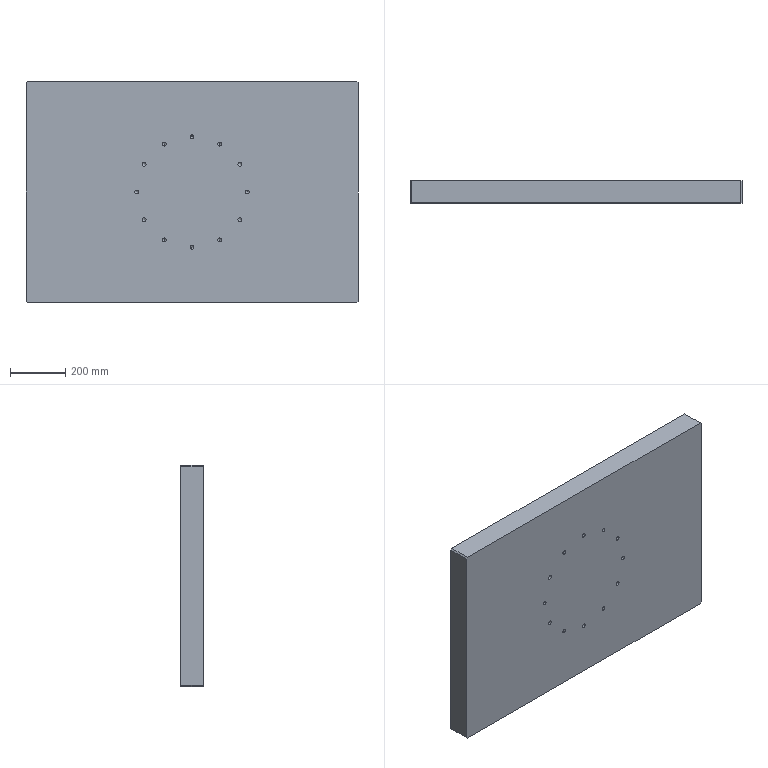Part | SolidWorks | features Chamfer 1, Extrusion 1, HoleWzd 1 | 1 solid | 58 faces | box 1200 x 80 x 800 mm | volume 76723214 mm3 | cylinder 24 | cone 24 | plane 10 | commonest cylinder face diameters 14 x24
STEP:
#1=CARTESIAN_POINT('',(0.,38.,207.));
#2=VERTEX_POINT('',#1);
#3=CARTESIAN_POINT('',(0.,38.,193.));
#4=VERTEX_POINT('',#3);
#5=CARTESIAN_POINT('',(0.,38.,200.));
#6=DIRECTION('',(0.,-1.,0.));
#7=DIRECTION('',(0.,0.,-1.));
#8=AXIS2_PLACEMENT_3D('',#5,#6,#7);
#9=CIRCLE('',#8,7.);
#10=EDGE_CURVE('',#2,#4,#9,.T.);
#11=ORIENTED_EDGE('',*,*,#10,.F.);
#12=CARTESIAN_POINT('',(0.,0.,207.));
#13=VERTEX_POINT('',#12);
#14=CARTESIAN_POINT('',(0.,0.,207.));
#15=DIRECTION('',(0.,-1.,0.));
#16=VECTOR('',#15,1000.);
#17=LINE('',#14,#16);
#18=EDGE_CURVE('',#2,#13,#17,.T.);
#19=ORIENTED_EDGE('',*,*,#18,.T.);
#20=CARTESIAN_POINT('',(0.,0.,193.));
#21=VERTEX_POINT('',#20);
#22=CARTESIAN_POINT('',(0.,0.,200.));
#23=DIRECTION('',(0.,-1.,0.));
#24=DIRECTION('',(0.,0.,-1.));
#25=AXIS2_PLACEMENT_3D('',#22,#23,#24);
#26=CIRCLE('',#25,7.);
#27=EDGE_CURVE('',#13,#21,#26,.T.);
#28=ORIENTED_EDGE('',*,*,#27,.T.);
#29=CARTESIAN_POINT('',(0.,0.,193.));
#30=DIRECTION('',(0.,-1.,0.));
#31=VECTOR('',#30,1000.);
#32=LINE('',#29,#31);
#33=EDGE_CURVE('',#4,#21,#32,.T.);
#34=ORIENTED_EDGE('',*,*,#33,.F.);
#35=EDGE_LOOP('',(#11,#19,#28,#34));
#36=FACE_OUTER_BOUND('',#35,.T.);
#37=CARTESIAN_POINT('',(0.,0.,200.));
#38=DIRECTION('',(0.,-1.,0.));
#39=DIRECTION('',(0.,0.,-1.));
#40=AXIS2_PLACEMENT_3D('',#37,#38,#39);
#41=CYLINDRICAL_SURFACE('',#40,7.);
#42=ADVANCED_FACE('',(#36),#41,.F.);
#43=CARTESIAN_POINT('',(0.,42.206,200.));
#44=VERTEX_POINT('',#43);
#45=CARTESIAN_POINT('',(0.,38.,193.));
#46=DIRECTION('',(0.,-0.515,-0.8572));
#47=VECTOR('',#46,1000.);
#48=LINE('',#45,#47);
#49=EDGE_CURVE('',#44,#4,#48,.T.);
#50=ORIENTED_EDGE('',*,*,#49,.F.);
#51=CARTESIAN_POINT('',(0.,38.,207.));
#52=DIRECTION('',(0.,-0.515,0.8572));
#53=VECTOR('',#52,1000.);
#54=LINE('',#51,#53);
#55=EDGE_CURVE('',#44,#2,#54,.T.);
#56=ORIENTED_EDGE('',*,*,#55,.T.);
#57=ORIENTED_EDGE('',*,*,#10,.T.);
#58=EDGE_LOOP('',(#50,#56,#57));
#59=FACE_OUTER_BOUND('',#58,.T.);
#60=CARTESIAN_POINT('',(0.,38.,200.));
#61=DIRECTION('',(0.,-1.,0.));
#62=DIRECTION('',(0.,0.,-1.));
#63=AXIS2_PLACEMENT_3D('',#60,#61,#62);
#64=CONICAL_SURFACE('',#63,7.,1.03);
#65=ADVANCED_FACE('',(#59),#64,.F.);
#66=CARTESIAN_POINT('',(-100.,38.,180.205));
#67=VERTEX_POINT('',#66);
#68=CARTESIAN_POINT('',(-100.,38.,166.205));
#69=VERTEX_POINT('',#68);
#70=CARTESIAN_POINT('',(-100.,38.,173.205));
#71=DIRECTION('',(0.,-1.,0.));
#72=DIRECTION('',(0.,0.,-1.));
#73=AXIS2_PLACEMENT_3D('',#70,#71,#72);
#74=CIRCLE('',#73,7.);
#75=EDGE_CURVE('',#67,#69,#74,.T.);
#76=ORIENTED_EDGE('',*,*,#75,.F.);
#77=CARTESIAN_POINT('',(-100.,0.,180.205));
#78=VERTEX_POINT('',#77);
#79=CARTESIAN_POINT('',(-100.,0.,180.205));
#80=DIRECTION('',(0.,-1.,0.));
#81=VECTOR('',#80,1000.);
#82=LINE('',#79,#81);
#83=EDGE_CURVE('',#67,#78,#82,.T.);
#84=ORIENTED_EDGE('',*,*,#83,.T.);
#85=CARTESIAN_POINT('',(-100.,0.,166.205));
#86=VERTEX_POINT('',#85);
#87=CARTESIAN_POINT('',(-100.,0.,173.205));
#88=DIRECTION('',(0.,-1.,0.));
#89=DIRECTION('',(0.,0.,-1.));
#90=AXIS2_PLACEMENT_3D('',#87,#88,#89);
#91=CIRCLE('',#90,7.);
#92=EDGE_CURVE('',#78,#86,#91,.T.);
#93=ORIENTED_EDGE('',*,*,#92,.T.);
#94=CARTESIAN_POINT('',(-100.,0.,166.205));
#95=DIRECTION('',(0.,-1.,0.));
#96=VECTOR('',#95,1000.);
#97=LINE('',#94,#96);
#98=EDGE_CURVE('',#69,#86,#97,.T.);
#99=ORIENTED_EDGE('',*,*,#98,.F.);
#100=EDGE_LOOP('',(#76,#84,#93,#99));
#101=FACE_OUTER_BOUND('',#100,.T.);
#102=CARTESIAN_POINT('',(-100.,0.,173.205));
#103=DIRECTION('',(0.,-1.,0.));
#104=DIRECTION('',(0.,0.,-1.));
#105=AXIS2_PLACEMENT_3D('',#102,#103,#104);
#106=CYLINDRICAL_SURFACE('',#105,7.);
#107=ADVANCED_FACE('',(#101),#106,.F.);
#108=CARTESIAN_POINT('',(-100.,42.206,173.205));
#109=VERTEX_POINT('',#108);
#110=CARTESIAN_POINT('',(-100.,38.,166.205));
#111=DIRECTION('',(0.,-0.515,-0.8572));
#112=VECTOR('',#111,1000.);
#113=LINE('',#110,#112);
#114=EDGE_CURVE('',#109,#69,#113,.T.);
#115=ORIENTED_EDGE('',*,*,#114,.F.);
#116=CARTESIAN_POINT('',(-100.,38.,180.205));
#117=DIRECTION('',(0.,-0.515,0.8572));
#118=VECTOR('',#117,1000.);
#119=LINE('',#116,#118);
#120=EDGE_CURVE('',#109,#67,#119,.T.);
#121=ORIENTED_EDGE('',*,*,#120,.T.);
#122=ORIENTED_EDGE('',*,*,#75,.T.);
#123=EDGE_LOOP('',(#115,#121,#122));
#124=FACE_OUTER_BOUND('',#123,.T.);
#125=CARTESIAN_POINT('',(-100.,38.,173.205));
#126=DIRECTION('',(0.,-1.,0.));
#127=DIRECTION('',(0.,0.,-1.));
#128=AXIS2_PLACEMENT_3D('',#125,#126,#127);
#129=CONICAL_SURFACE('',#128,7.,1.03);
#130=ADVANCED_FACE('',(#124),#129,.F.);
#131=CARTESIAN_POINT('',(-173.205,38.,107.));
#132=VERTEX_POINT('',#131);
#133=CARTESIAN_POINT('',(-173.205,38.,93.));
#134=VERTEX_POINT('',#133);
#135=CARTESIAN_POINT('',(-173.205,38.,100.));
#136=DIRECTION('',(0.,-1.,0.));
#137=DIRECTION('',(0.,0.,-1.));
#138=AXIS2_PLACEMENT_3D('',#135,#136,#137);
#139=CIRCLE('',#138,7.);
#140=EDGE_CURVE('',#132,#134,#139,.T.);
#141=ORIENTED_EDGE('',*,*,#140,.F.);
#142=CARTESIAN_POINT('',(-173.205,0.,107.));
#143=VERTEX_POINT('',#142);
#144=CARTESIAN_POINT('',(-173.205,0.,107.));
#145=DIRECTION('',(0.,-1.,0.));
#146=VECTOR('',#145,1000.);
#147=LINE('',#144,#146);
#148=EDGE_CURVE('',#132,#143,#147,.T.);
#149=ORIENTED_EDGE('',*,*,#148,.T.);
#150=CARTESIAN_POINT('',(-173.205,0.,93.));
#151=VERTEX_POINT('',#150);
#152=CARTESIAN_POINT('',(-173.205,0.,100.));
#153=DIRECTION('',(0.,-1.,0.));
#154=DIRECTION('',(0.,0.,-1.));
#155=AXIS2_PLACEMENT_3D('',#152,#153,#154);
#156=CIRCLE('',#155,7.);
#157=EDGE_CURVE('',#143,#151,#156,.T.);
#158=ORIENTED_EDGE('',*,*,#157,.T.);
#159=CARTESIAN_POINT('',(-173.205,0.,93.));
#160=DIRECTION('',(0.,-1.,0.));
#161=VECTOR('',#160,1000.);
#162=LINE('',#159,#161);
#163=EDGE_CURVE('',#134,#151,#162,.T.);
#164=ORIENTED_EDGE('',*,*,#163,.F.);
#165=EDGE_LOOP('',(#141,#149,#158,#164));
#166=FACE_OUTER_BOUND('',#165,.T.);
#167=CARTESIAN_POINT('',(-173.205,0.,100.));
#168=DIRECTION('',(0.,-1.,0.));
#169=DIRECTION('',(0.,0.,-1.));
#170=AXIS2_PLACEMENT_3D('',#167,#168,#169);
#171=CYLINDRICAL_SURFACE('',#170,7.);
#172=ADVANCED_FACE('',(#166),#171,.F.);
#173=CARTESIAN_POINT('',(-173.205,42.206,100.));
#174=VERTEX_POINT('',#173);
#175=CARTESIAN_POINT('',(-173.205,38.,93.));
#176=DIRECTION('',(0.,-0.515,-0.8572));
#177=VECTOR('',#176,1000.);
#178=LINE('',#175,#177);
#179=EDGE_CURVE('',#174,#134,#178,.T.);
#180=ORIENTED_EDGE('',*,*,#179,.F.);
#181=CARTESIAN_POINT('',(-173.205,38.,107.));
#182=DIRECTION('',(0.,-0.515,0.8572));
#183=VECTOR('',#182,1000.);
#184=LINE('',#181,#183);
#185=EDGE_CURVE('',#174,#132,#184,.T.);
#186=ORIENTED_EDGE('',*,*,#185,.T.);
#187=ORIENTED_EDGE('',*,*,#140,.T.);
#188=EDGE_LOOP('',(#180,#186,#187));
#189=FACE_OUTER_BOUND('',#188,.T.);
#190=CARTESIAN_POINT('',(-173.205,38.,100.));
#191=DIRECTION('',(0.,-1.,0.));
#192=DIRECTION('',(0.,0.,-1.));
#193=AXIS2_PLACEMENT_3D('',#190,#191,#192);
#194=CONICAL_SURFACE('',#193,7.,1.03);
#195=ADVANCED_FACE('',(#189),#194,.F.);
#196=CARTESIAN_POINT('',(-200.,38.,7.));
#197=VERTEX_POINT('',#196);
#198=CARTESIAN_POINT('',(-200.,38.,-7.));
#199=VERTEX_POINT('',#198);
#200=CARTESIAN_POINT('',(-200.,38.,0.));
#201=DIRECTION('',(0.,-1.,0.));
#202=DIRECTION('',(0.,0.,-1.));
#203=AXIS2_PLACEMENT_3D('',#200,#201,#202);
#204=CIRCLE('',#203,7.);
#205=EDGE_CURVE('',#197,#199,#204,.T.);
#206=ORIENTED_EDGE('',*,*,#205,.F.);
#207=CARTESIAN_POINT('',(-200.,0.,7.));
#208=VERTEX_POINT('',#207);
#209=CARTESIAN_POINT('',(-200.,0.,7.));
#210=DIRECTION('',(0.,-1.,0.));
#211=VECTOR('',#210,1000.);
#212=LINE('',#209,#211);
#213=EDGE_CURVE('',#197,#208,#212,.T.);
#214=ORIENTED_EDGE('',*,*,#213,.T.);
#215=CARTESIAN_POINT('',(-200.,0.,-7.));
#216=VERTEX_POINT('',#215);
#217=CARTESIAN_POINT('',(-200.,0.,0.));
#218=DIRECTION('',(0.,-1.,0.));
#219=DIRECTION('',(0.,0.,-1.));
#220=AXIS2_PLACEMENT_3D('',#217,#218,#219);
#221=CIRCLE('',#220,7.);
#222=EDGE_CURVE('',#208,#216,#221,.T.);
#223=ORIENTED_EDGE('',*,*,#222,.T.);
#224=CARTESIAN_POINT('',(-200.,0.,-7.));
#225=DIRECTION('',(0.,-1.,0.));
#226=VECTOR('',#225,1000.);
#227=LINE('',#224,#226);
#228=EDGE_CURVE('',#199,#216,#227,.T.);
#229=ORIENTED_EDGE('',*,*,#228,.F.);
#230=EDGE_LOOP('',(#206,#214,#223,#229));
#231=FACE_OUTER_BOUND('',#230,.T.);
#232=CARTESIAN_POINT('',(-200.,0.,0.));
#233=DIRECTION('',(0.,-1.,0.));
#234=DIRECTION('',(0.,0.,-1.));
#235=AXIS2_PLACEMENT_3D('',#232,#233,#234);
#236=CYLINDRICAL_SURFACE('',#235,7.);
#237=ADVANCED_FACE('',(#231),#236,.F.);
#238=CARTESIAN_POINT('',(-200.,42.206,0.));
#239=VERTEX_POINT('',#238);
#240=CARTESIAN_POINT('',(-200.,38.,-7.));
#241=DIRECTION('',(0.,-0.515,-0.8572));
#242=VECTOR('',#241,1000.);
#243=LINE('',#240,#242);
#244=EDGE_CURVE('',#239,#199,#243,.T.);
#245=ORIENTED_EDGE('',*,*,#244,.F.);
#246=CARTESIAN_POINT('',(-200.,38.,7.));
#247=DIRECTION('',(0.,-0.515,0.8572));
#248=VECTOR('',#247,1000.);
#249=LINE('',#246,#248);
#250=EDGE_CURVE('',#239,#197,#249,.T.);
#251=ORIENTED_EDGE('',*,*,#250,.T.);
#252=ORIENTED_EDGE('',*,*,#205,.T.);
#253=EDGE_LOOP('',(#245,#251,#252));
#254=FACE_OUTER_BOUND('',#253,.T.);
#255=CARTESIAN_POINT('',(-200.,38.,0.));
#256=DIRECTION('',(0.,-1.,0.));
#257=DIRECTION('',(0.,0.,-1.));
#258=AXIS2_PLACEMENT_3D('',#255,#256,#257);
#259=CONICAL_SURFACE('',#258,7.,1.03);
#260=ADVANCED_FACE('',(#254),#259,.F.);
#261=CARTESIAN_POINT('',(-173.205,38.,-93.));
#262=VERTEX_POINT('',#261);
#263=CARTESIAN_POINT('',(-173.205,38.,-107.));
#264=VERTEX_POINT('',#263);
#265=CARTESIAN_POINT('',(-173.205,38.,-100.));
#266=DIRECTION('',(0.,-1.,0.));
#267=DIRECTION('',(0.,0.,-1.));
#268=AXIS2_PLACEMENT_3D('',#265,#266,#267);
#269=CIRCLE('',#268,7.);
#270=EDGE_CURVE('',#262,#264,#269,.T.);
#271=ORIENTED_EDGE('',*,*,#270,.F.);
#272=CARTESIAN_POINT('',(-173.205,0.,-93.));
#273=VERTEX_POINT('',#272);
#274=CARTESIAN_POINT('',(-173.205,0.,-93.));
#275=DIRECTION('',(0.,-1.,0.));
#276=VECTOR('',#275,1000.);
#277=LINE('',#274,#276);
#278=EDGE_CURVE('',#262,#273,#277,.T.);
#279=ORIENTED_EDGE('',*,*,#278,.T.);
#280=CARTESIAN_POINT('',(-173.205,0.,-107.));
#281=VERTEX_POINT('',#280);
#282=CARTESIAN_POINT('',(-173.205,0.,-100.));
#283=DIRECTION('',(0.,-1.,0.));
#284=DIRECTION('',(0.,0.,-1.));
#285=AXIS2_PLACEMENT_3D('',#282,#283,#284);
#286=CIRCLE('',#285,7.);
#287=EDGE_CURVE('',#273,#281,#286,.T.);
#288=ORIENTED_EDGE('',*,*,#287,.T.);
#289=CARTESIAN_POINT('',(-173.205,0.,-107.));
#290=DIRECTION('',(0.,-1.,0.));
#291=VECTOR('',#290,1000.);
#292=LINE('',#289,#291);
#293=EDGE_CURVE('',#264,#281,#292,.T.);
#294=ORIENTED_EDGE('',*,*,#293,.F.);
#295=EDGE_LOOP('',(#271,#279,#288,#294));
#296=FACE_OUTER_BOUND('',#295,.T.);
#297=CARTESIAN_POINT('',(-173.205,0.,-100.));
#298=DIRECTION('',(0.,-1.,0.));
#299=DIRECTION('',(0.,0.,-1.));
#300=AXIS2_PLACEMENT_3D('',#297,#298,#299);
#301=CYLINDRICAL_SURFACE('',#300,7.);
#302=ADVANCED_FACE('',(#296),#301,.F.);
#303=CARTESIAN_POINT('',(-173.205,42.206,-100.));
#304=VERTEX_POINT('',#303);
#305=CARTESIAN_POINT('',(-173.205,38.,-107.));
#306=DIRECTION('',(0.,-0.515,-0.8572));
#307=VECTOR('',#306,1000.);
#308=LINE('',#305,#307);
#309=EDGE_CURVE('',#304,#264,#308,.T.);
#310=ORIENTED_EDGE('',*,*,#309,.F.);
#311=CARTESIAN_POINT('',(-173.205,38.,-93.));
#312=DIRECTION('',(0.,-0.515,0.8572));
#313=VECTOR('',#312,1000.);
#314=LINE('',#311,#313);
#315=EDGE_CURVE('',#304,#262,#314,.T.);
#316=ORIENTED_EDGE('',*,*,#315,.T.);
#317=ORIENTED_EDGE('',*,*,#270,.T.);
#318=EDGE_LOOP('',(#310,#316,#317));
#319=FACE_OUTER_BOUND('',#318,.T.);
#320=CARTESIAN_POINT('',(-173.205,38.,-100.));
#321=DIRECTION('',(0.,-1.,0.));
#322=DIRECTION('',(0.,0.,-1.));
#323=AXIS2_PLACEMENT_3D('',#320,#321,#322);
#324=CONICAL_SURFACE('',#323,7.,1.03);
#325=ADVANCED_FACE('',(#319),#324,.F.);
#326=CARTESIAN_POINT('',(-100.,38.,-166.205));
#327=VERTEX_POINT('',#326);
#328=CARTESIAN_POINT('',(-100.,38.,-180.205));
#329=VERTEX_POINT('',#328);
#330=CARTESIAN_POINT('',(-100.,38.,-173.205));
#331=DIRECTION('',(0.,-1.,0.));
#332=DIRECTION('',(0.,0.,-1.));
#333=AXIS2_PLACEMENT_3D('',#330,#331,#332);
#334=CIRCLE('',#333,7.);
#335=EDGE_CURVE('',#327,#329,#334,.T.);
#336=ORIENTED_EDGE('',*,*,#335,.F.);
#337=CARTESIAN_POINT('',(-100.,0.,-166.205));
#338=VERTEX_POINT('',#337);
#339=CARTESIAN_POINT('',(-100.,0.,-166.205));
#340=DIRECTION('',(0.,-1.,0.));
#341=VECTOR('',#340,1000.);
#342=LINE('',#339,#341);
#343=EDGE_CURVE('',#327,#338,#342,.T.);
#344=ORIENTED_EDGE('',*,*,#343,.T.);
#345=CARTESIAN_POINT('',(-100.,0.,-180.205));
#346=VERTEX_POINT('',#345);
#347=CARTESIAN_POINT('',(-100.,0.,-173.205));
#348=DIRECTION('',(0.,-1.,0.));
#349=DIRECTION('',(0.,0.,-1.));
#350=AXIS2_PLACEMENT_3D('',#347,#348,#349);
#351=CIRCLE('',#350,7.);
#352=EDGE_CURVE('',#338,#346,#351,.T.);
#353=ORIENTED_EDGE('',*,*,#352,.T.);
#354=CARTESIAN_POINT('',(-100.,0.,-180.205));
#355=DIRECTION('',(0.,-1.,0.));
#356=VECTOR('',#355,1000.);
#357=LINE('',#354,#356);
#358=EDGE_CURVE('',#329,#346,#357,.T.);
#359=ORIENTED_EDGE('',*,*,#358,.F.);
#360=EDGE_LOOP('',(#336,#344,#353,#359));
#361=FACE_OUTER_BOUND('',#360,.T.);
#362=CARTESIAN_POINT('',(-100.,0.,-173.205));
#363=DIRECTION('',(0.,-1.,0.));
#364=DIRECTION('',(0.,0.,-1.));
#365=AXIS2_PLACEMENT_3D('',#362,#363,#364);
#366=CYLINDRICAL_SURFACE('',#365,7.);
#367=ADVANCED_FACE('',(#361),#366,.F.);
#368=CARTESIAN_POINT('',(-100.,42.206,-173.205));
#369=VERTEX_POINT('',#368);
#370=CARTESIAN_POINT('',(-100.,38.,-180.205));
#371=DIRECTION('',(0.,-0.515,-0.8572));
#372=VECTOR('',#371,1000.);
#373=LINE('',#370,#372);
#374=EDGE_CURVE('',#369,#329,#373,.T.);
#375=ORIENTED_EDGE('',*,*,#374,.F.);
#376=CARTESIAN_POINT('',(-100.,38.,-166.205));
#377=DIRECTION('',(0.,-0.515,0.8572));
#378=VECTOR('',#377,1000.);
#379=LINE('',#376,#378);
#380=EDGE_CURVE('',#369,#327,#379,.T.);
#381=ORIENTED_EDGE('',*,*,#380,.T.);
#382=ORIENTED_EDGE('',*,*,#335,.T.);
#383=EDGE_LOOP('',(#375,#381,#382));
#384=FACE_OUTER_BOUND('',#383,.T.);
#385=CARTESIAN_POINT('',(-100.,38.,-173.205));
#386=DIRECTION('',(0.,-1.,0.));
#387=DIRECTION('',(0.,0.,-1.));
#388=AXIS2_PLACEMENT_3D('',#385,#386,#387);
#389=CONICAL_SURFACE('',#388,7.,1.03);
#390=ADVANCED_FACE('',(#384),#389,.F.);
#391=CARTESIAN_POINT('',(0.,38.,-193.));
#392=VERTEX_POINT('',#391);
#393=CARTESIAN_POINT('',(0.,38.,-207.));
#394=VERTEX_POINT('',#393);
#395=CARTESIAN_POINT('',(0.,38.,-200.));
#396=DIRECTION('',(0.,-1.,0.));
#397=DIRECTION('',(0.,0.,-1.));
#398=AXIS2_PLACEMENT_3D('',#395,#396,#397);
#399=CIRCLE('',#398,7.);
#400=EDGE_CURVE('',#392,#394,#399,.T.);
#401=ORIENTED_EDGE('',*,*,#400,.F.);
#402=CARTESIAN_POINT('',(0.,0.,-193.));
#403=VERTEX_POINT('',#402);
#404=CARTESIAN_POINT('',(0.,0.,-193.));
#405=DIRECTION('',(0.,-1.,0.));
#406=VECTOR('',#405,1000.);
#407=LINE('',#404,#406);
#408=EDGE_CURVE('',#392,#403,#407,.T.);
#409=ORIENTED_EDGE('',*,*,#408,.T.);
#410=CARTESIAN_POINT('',(0.,0.,-207.));
#411=VERTEX_POINT('',#410);
#412=CARTESIAN_POINT('',(0.,0.,-200.));
#413=DIRECTION('',(0.,-1.,0.));
#414=DIRECTION('',(0.,0.,-1.));
#415=AXIS2_PLACEMENT_3D('',#412,#413,#414);
#416=CIRCLE('',#415,7.);
#417=EDGE_CURVE('',#403,#411,#416,.T.);
#418=ORIENTED_EDGE('',*,*,#417,.T.);
#419=CARTESIAN_POINT('',(0.,0.,-207.));
#420=DIRECTION('',(0.,-1.,0.));
#421=VECTOR('',#420,1000.);
#422=LINE('',#419,#421);
#423=EDGE_CURVE('',#394,#411,#422,.T.);
#424=ORIENTED_EDGE('',*,*,#423,.F.);
#425=EDGE_LOOP('',(#401,#409,#418,#424));
#426=FACE_OUTER_BOUND('',#425,.T.);
#427=CARTESIAN_POINT('',(0.,0.,-200.));
#428=DIRECTION('',(0.,-1.,0.));
#429=DIRECTION('',(0.,0.,-1.));
#430=AXIS2_PLACEMENT_3D('',#427,#428,#429);
#431=CYLINDRICAL_SURFACE('',#430,7.);
#432=ADVANCED_FACE('',(#426),#431,.F.);
#433=CARTESIAN_POINT('',(0.,42.206,-200.));
#434=VERTEX_POINT('',#433);
#435=CARTESIAN_POINT('',(0.,38.,-207.));
#436=DIRECTION('',(0.,-0.515,-0.8572));
#437=VECTOR('',#436,1000.);
#438=LINE('',#435,#437);
#439=EDGE_CURVE('',#434,#394,#438,.T.);
#440=ORIENTED_EDGE('',*,*,#439,.F.);
#441=CARTESIAN_POINT('',(0.,38.,-193.));
#442=DIRECTION('',(0.,-0.515,0.8572));
#443=VECTOR('',#442,1000.);
#444=LINE('',#441,#443);
#445=EDGE_CURVE('',#434,#392,#444,.T.);
#446=ORIENTED_EDGE('',*,*,#445,.T.);
#447=ORIENTED_EDGE('',*,*,#400,.T.);
#448=EDGE_LOOP('',(#440,#446,#447));
#449=FACE_OUTER_BOUND('',#448,.T.);
#450=CARTESIAN_POINT('',(0.,38.,-200.));
#451=DIRECTION('',(0.,-1.,0.));
#452=DIRECTION('',(0.,0.,-1.));
#453=AXIS2_PLACEMENT_3D('',#450,#451,#452);
#454=CONICAL_SURFACE('',#453,7.,1.03);
#455=ADVANCED_FACE('',(#449),#454,.F.);
#456=CARTESIAN_POINT('',(100.,38.,-166.205));
#457=VERTEX_POINT('',#456);
#458=CARTESIAN_POINT('',(100.,38.,-180.205));
#459=VERTEX_POINT('',#458);
#460=CARTESIAN_POINT('',(100.,38.,-173.205));
#461=DIRECTION('',(0.,-1.,0.));
#462=DIRECTION('',(0.,0.,-1.));
#463=AXIS2_PLACEMENT_3D('',#460,#461,#462);
#464=CIRCLE('',#463,7.);
#465=EDGE_CURVE('',#457,#459,#464,.T.);
#466=ORIENTED_EDGE('',*,*,#465,.F.);
#467=CARTESIAN_POINT('',(100.,0.,-166.205));
#468=VERTEX_POINT('',#467);
#469=CARTESIAN_POINT('',(100.,0.,-166.205));
#470=DIRECTION('',(0.,-1.,0.));
#471=VECTOR('',#470,1000.);
#472=LINE('',#469,#471);
#473=EDGE_CURVE('',#457,#468,#472,.T.);
#474=ORIENTED_EDGE('',*,*,#473,.T.);
#475=CARTESIAN_POINT('',(100.,0.,-180.205));
#476=VERTEX_POINT('',#475);
#477=CARTESIAN_POINT('',(100.,0.,-173.205));
#478=DIRECTION('',(0.,-1.,0.));
#479=DIRECTION('',(0.,0.,-1.));
#480=AXIS2_PLACEMENT_3D('',#477,#478,#479);
#481=CIRCLE('',#480,7.);
#482=EDGE_CURVE('',#468,#476,#481,.T.);
#483=ORIENTED_EDGE('',*,*,#482,.T.);
#484=CARTESIAN_POINT('',(100.,0.,-180.205));
#485=DIRECTION('',(0.,-1.,0.));
#486=VECTOR('',#485,1000.);
#487=LINE('',#484,#486);
#488=EDGE_CURVE('',#459,#476,#487,.T.);
#489=ORIENTED_EDGE('',*,*,#488,.F.);
#490=EDGE_LOOP('',(#466,#474,#483,#489));
#491=FACE_OUTER_BOUND('',#490,.T.);
#492=CARTESIAN_POINT('',(100.,0.,-173.205));
#493=DIRECTION('',(0.,-1.,0.));
#494=DIRECTION('',(0.,0.,-1.));
#495=AXIS2_PLACEMENT_3D('',#492,#493,#494);
#496=CYLINDRICAL_SURFACE('',#495,7.);
#497=ADVANCED_FACE('',(#491),#496,.F.);
#498=CARTESIAN_POINT('',(100.,42.206,-173.205));
#499=VERTEX_POINT('',#498);
#500=CARTESIAN_POINT('',(100.,38.,-180.205));
#501=DIRECTION('',(0.,-0.515,-0.8572));
#502=VECTOR('',#501,1000.);
#503=LINE('',#500,#502);
#504=EDGE_CURVE('',#499,#459,#503,.T.);
#505=ORIENTED_EDGE('',*,*,#504,.F.);
#506=CARTESIAN_POINT('',(100.,38.,-166.205));
#507=DIRECTION('',(0.,-0.515,0.8572));
#508=VECTOR('',#507,1000.);
#509=LINE('',#506,#508);
#510=EDGE_CURVE('',#499,#457,#509,.T.);
#511=ORIENTED_EDGE('',*,*,#510,.T.);
#512=ORIENTED_EDGE('',*,*,#465,.T.);
#513=EDGE_LOOP('',(#505,#511,#512));
#514=FACE_OUTER_BOUND('',#513,.T.);
#515=CARTESIAN_POINT('',(100.,38.,-173.205));
#516=DIRECTION('',(0.,-1.,0.));
#517=DIRECTION('',(0.,0.,-1.));
#518=AXIS2_PLACEMENT_3D('',#515,#516,#517);
#519=CONICAL_SURFACE('',#518,7.,1.03);
#520=ADVANCED_FACE('',(#514),#519,.F.);
#521=CARTESIAN_POINT('',(173.205,38.,-93.));
#522=VERTEX_POINT('',#521);
#523=CARTESIAN_POINT('',(173.205,38.,-107.));
#524=VERTEX_POINT('',#523);
#525=CARTESIAN_POINT('',(173.205,38.,-100.));
#526=DIRECTION('',(0.,-1.,0.));
#527=DIRECTION('',(0.,0.,-1.));
#528=AXIS2_PLACEMENT_3D('',#525,#526,#527);
#529=CIRCLE('',#528,7.);
#530=EDGE_CURVE('',#522,#524,#529,.T.);
#531=ORIENTED_EDGE('',*,*,#530,.F.);
#532=CARTESIAN_POINT('',(173.205,0.,-93.));
#533=VERTEX_POINT('',#532);
#534=CARTESIAN_POINT('',(173.205,0.,-93.));
#535=DIRECTION('',(0.,-1.,0.));
#536=VECTOR('',#535,1000.);
#537=LINE('',#534,#536);
#538=EDGE_CURVE('',#522,#533,#537,.T.);
#539=ORIENTED_EDGE('',*,*,#538,.T.);
#540=CARTESIAN_POINT('',(173.205,0.,-107.));
#541=VERTEX_POINT('',#540);
#542=CARTESIAN_POINT('',(173.205,0.,-100.));
#543=DIRECTION('',(0.,-1.,0.));
#544=DIRECTION('',(0.,0.,-1.));
#545=AXIS2_PLACEMENT_3D('',#542,#543,#544);
#546=CIRCLE('',#545,7.);
#547=EDGE_CURVE('',#533,#541,#546,.T.);
#548=ORIENTED_EDGE('',*,*,#547,.T.);
#549=CARTESIAN_POINT('',(173.205,0.,-107.));
#550=DIRECTION('',(0.,-1.,0.));
#551=VECTOR('',#550,1000.);
#552=LINE('',#549,#551);
#553=EDGE_CURVE('',#524,#541,#552,.T.);
#554=ORIENTED_EDGE('',*,*,#553,.F.);
#555=EDGE_LOOP('',(#531,#539,#548,#554));
#556=FACE_OUTER_BOUND('',#555,.T.);
#557=CARTESIAN_POINT('',(173.205,0.,-100.));
#558=DIRECTION('',(0.,-1.,0.));
#559=DIRECTION('',(0.,0.,-1.));
#560=AXIS2_PLACEMENT_3D('',#557,#558,#559);
#561=CYLINDRICAL_SURFACE('',#560,7.);
#562=ADVANCED_FACE('',(#556),#561,.F.);
#563=CARTESIAN_POINT('',(173.205,42.206,-100.));
#564=VERTEX_POINT('',#563);
#565=CARTESIAN_POINT('',(173.205,38.,-107.));
#566=DIRECTION('',(0.,-0.515,-0.8572));
#567=VECTOR('',#566,1000.);
#568=LINE('',#565,#567);
#569=EDGE_CURVE('',#564,#524,#568,.T.);
#570=ORIENTED_EDGE('',*,*,#569,.F.);
#571=CARTESIAN_POINT('',(173.205,38.,-93.));
#572=DIRECTION('',(0.,-0.515,0.8572));
#573=VECTOR('',#572,1000.);
#574=LINE('',#571,#573);
#575=EDGE_CURVE('',#564,#522,#574,.T.);
#576=ORIENTED_EDGE('',*,*,#575,.T.);
#577=ORIENTED_EDGE('',*,*,#530,.T.);
#578=EDGE_LOOP('',(#570,#576,#577));
#579=FACE_OUTER_BOUND('',#578,.T.);
#580=CARTESIAN_POINT('',(173.205,38.,-100.));
#581=DIRECTION('',(0.,-1.,0.));
#582=DIRECTION('',(0.,0.,-1.));
#583=AXIS2_PLACEMENT_3D('',#580,#581,#582);
#584=CONICAL_SURFACE('',#583,7.,1.03);
#585=ADVANCED_FACE('',(#579),#584,.F.);
#586=CARTESIAN_POINT('',(200.,38.,7.));
#587=VERTEX_POINT('',#586);
#588=CARTESIAN_POINT('',(200.,38.,-7.));
#589=VERTEX_POINT('',#588);
#590=CARTESIAN_POINT('',(200.,38.,0.));
#591=DIRECTION('',(0.,-1.,0.));
#592=DIRECTION('',(0.,0.,-1.));
#593=AXIS2_PLACEMENT_3D('',#590,#591,#592);
#594=CIRCLE('',#593,7.);
#595=EDGE_CURVE('',#587,#589,#594,.T.);
#596=ORIENTED_EDGE('',*,*,#595,.F.);
#597=CARTESIAN_POINT('',(200.,0.,7.));
#598=VERTEX_POINT('',#597);
#599=CARTESIAN_POINT('',(200.,0.,7.));
#600=DIRECTION('',(0.,-1.,0.));
#601=VECTOR('',#600,1000.);
#602=LINE('',#599,#601);
#603=EDGE_CURVE('',#587,#598,#602,.T.);
#604=ORIENTED_EDGE('',*,*,#603,.T.);
#605=CARTESIAN_POINT('',(200.,0.,-7.));
#606=VERTEX_POINT('',#605);
#607=CARTESIAN_POINT('',(200.,0.,0.));
#608=DIRECTION('',(0.,-1.,0.));
#609=DIRECTION('',(0.,0.,-1.));
#610=AXIS2_PLACEMENT_3D('',#607,#608,#609);
#611=CIRCLE('',#610,7.);
#612=EDGE_CURVE('',#598,#606,#611,.T.);
#613=ORIENTED_EDGE('',*,*,#612,.T.);
#614=CARTESIAN_POINT('',(200.,0.,-7.));
#615=DIRECTION('',(0.,-1.,0.));
#616=VECTOR('',#615,1000.);
#617=LINE('',#614,#616);
#618=EDGE_CURVE('',#589,#606,#617,.T.);
#619=ORIENTED_EDGE('',*,*,#618,.F.);
#620=EDGE_LOOP('',(#596,#604,#613,#619));
#621=FACE_OUTER_BOUND('',#620,.T.);
#622=CARTESIAN_POINT('',(200.,0.,0.));
#623=DIRECTION('',(0.,-1.,0.));
#624=DIRECTION('',(0.,0.,-1.));
#625=AXIS2_PLACEMENT_3D('',#622,#623,#624);
#626=CYLINDRICAL_SURFACE('',#625,7.);
#627=ADVANCED_FACE('',(#621),#626,.F.);
#628=CARTESIAN_POINT('',(200.,42.206,0.));
#629=VERTEX_POINT('',#628);
#630=CARTESIAN_POINT('',(200.,38.,-7.));
#631=DIRECTION('',(0.,-0.515,-0.8572));
#632=VECTOR('',#631,1000.);
#633=LINE('',#630,#632);
#634=EDGE_CURVE('',#629,#589,#633,.T.);
#635=ORIENTED_EDGE('',*,*,#634,.F.);
#636=CARTESIAN_POINT('',(200.,38.,7.));
#637=DIRECTION('',(0.,-0.515,0.8572));
#638=VECTOR('',#637,1000.);
#639=LINE('',#636,#638);
#640=EDGE_CURVE('',#629,#587,#639,.T.);
#641=ORIENTED_EDGE('',*,*,#640,.T.);
#642=ORIENTED_EDGE('',*,*,#595,.T.);
#643=EDGE_LOOP('',(#635,#641,#642));
#644=FACE_OUTER_BOUND('',#643,.T.);
#645=CARTESIAN_POINT('',(200.,38.,0.));
#646=DIRECTION('',(0.,-1.,0.));
#647=DIRECTION('',(0.,0.,-1.));
#648=AXIS2_PLACEMENT_3D('',#645,#646,#647);
#649=CONICAL_SURFACE('',#648,7.,1.03);
#650=ADVANCED_FACE('',(#644),#649,.F.);
#651=CARTESIAN_POINT('',(173.205,38.,107.));
#652=VERTEX_POINT('',#651);
#653=CARTESIAN_POINT('',(173.205,38.,93.));
#654=VERTEX_POINT('',#653);
#655=CARTESIAN_POINT('',(173.205,38.,100.));
#656=DIRECTION('',(0.,-1.,0.));
#657=DIRECTION('',(0.,0.,-1.));
#658=AXIS2_PLACEMENT_3D('',#655,#656,#657);
#659=CIRCLE('',#658,7.);
#660=EDGE_CURVE('',#652,#654,#659,.T.);
#661=ORIENTED_EDGE('',*,*,#660,.F.);
#662=CARTESIAN_POINT('',(173.205,0.,107.));
#663=VERTEX_POINT('',#662);
#664=CARTESIAN_POINT('',(173.205,0.,107.));
#665=DIRECTION('',(0.,-1.,0.));
#666=VECTOR('',#665,1000.);
#667=LINE('',#664,#666);
#668=EDGE_CURVE('',#652,#663,#667,.T.);
#669=ORIENTED_EDGE('',*,*,#668,.T.);
#670=CARTESIAN_POINT('',(173.205,0.,93.));
#671=VERTEX_POINT('',#670);
#672=CARTESIAN_POINT('',(173.205,0.,100.));
#673=DIRECTION('',(0.,-1.,0.));
#674=DIRECTION('',(0.,0.,-1.));
#675=AXIS2_PLACEMENT_3D('',#672,#673,#674);
#676=CIRCLE('',#675,7.);
#677=EDGE_CURVE('',#663,#671,#676,.T.);
#678=ORIENTED_EDGE('',*,*,#677,.T.);
#679=CARTESIAN_POINT('',(173.205,0.,93.));
#680=DIRECTION('',(0.,-1.,0.));
#681=VECTOR('',#680,1000.);
#682=LINE('',#679,#681);
#683=EDGE_CURVE('',#654,#671,#682,.T.);
#684=ORIENTED_EDGE('',*,*,#683,.F.);
#685=EDGE_LOOP('',(#661,#669,#678,#684));
#686=FACE_OUTER_BOUND('',#685,.T.);
#687=CARTESIAN_POINT('',(173.205,0.,100.));
#688=DIRECTION('',(0.,-1.,0.));
#689=DIRECTION('',(0.,0.,-1.));
#690=AXIS2_PLACEMENT_3D('',#687,#688,#689);
#691=CYLINDRICAL_SURFACE('',#690,7.);
#692=ADVANCED_FACE('',(#686),#691,.F.);
#693=CARTESIAN_POINT('',(173.205,42.206,100.));
#694=VERTEX_POINT('',#693);
#695=CARTESIAN_POINT('',(173.205,38.,93.));
#696=DIRECTION('',(0.,-0.515,-0.8572));
#697=VECTOR('',#696,1000.);
#698=LINE('',#695,#697);
#699=EDGE_CURVE('',#694,#654,#698,.T.);
#700=ORIENTED_EDGE('',*,*,#699,.F.);
#701=CARTESIAN_POINT('',(173.205,38.,107.));
#702=DIRECTION('',(0.,-0.515,0.8572));
#703=VECTOR('',#702,1000.);
#704=LINE('',#701,#703);
#705=EDGE_CURVE('',#694,#652,#704,.T.);
#706=ORIENTED_EDGE('',*,*,#705,.T.);
#707=ORIENTED_EDGE('',*,*,#660,.T.);
#708=EDGE_LOOP('',(#700,#706,#707));
#709=FACE_OUTER_BOUND('',#708,.T.);
#710=CARTESIAN_POINT('',(173.205,38.,100.));
#711=DIRECTION('',(0.,-1.,0.));
#712=DIRECTION('',(0.,0.,-1.));
#713=AXIS2_PLACEMENT_3D('',#710,#711,#712);
#714=CONICAL_SURFACE('',#713,7.,1.03);
#715=ADVANCED_FACE('',(#709),#714,.F.);
#716=CARTESIAN_POINT('',(100.,38.,180.205));
#717=VERTEX_POINT('',#716);
#718=CARTESIAN_POINT('',(100.,38.,166.205));
#719=VERTEX_POINT('',#718);
#720=CARTESIAN_POINT('',(100.,38.,173.205));
#721=DIRECTION('',(0.,-1.,0.));
#722=DIRECTION('',(0.,0.,-1.));
#723=AXIS2_PLACEMENT_3D('',#720,#721,#722);
#724=CIRCLE('',#723,7.);
#725=EDGE_CURVE('',#717,#719,#724,.T.);
#726=ORIENTED_EDGE('',*,*,#725,.F.);
#727=CARTESIAN_POINT('',(100.,0.,180.205));
#728=VERTEX_POINT('',#727);
#729=CARTESIAN_POINT('',(100.,0.,180.205));
#730=DIRECTION('',(0.,-1.,0.));
#731=VECTOR('',#730,1000.);
#732=LINE('',#729,#731);
#733=EDGE_CURVE('',#717,#728,#732,.T.);
#734=ORIENTED_EDGE('',*,*,#733,.T.);
#735=CARTESIAN_POINT('',(100.,0.,166.205));
#736=VERTEX_POINT('',#735);
#737=CARTESIAN_POINT('',(100.,0.,173.205));
#738=DIRECTION('',(0.,-1.,0.));
#739=DIRECTION('',(0.,0.,-1.));
#740=AXIS2_PLACEMENT_3D('',#737,#738,#739);
#741=CIRCLE('',#740,7.);
#742=EDGE_CURVE('',#728,#736,#741,.T.);
#743=ORIENTED_EDGE('',*,*,#742,.T.);
#744=CARTESIAN_POINT('',(100.,0.,166.205));
#745=DIRECTION('',(0.,-1.,0.));
#746=VECTOR('',#745,1000.);
#747=LINE('',#744,#746);
#748=EDGE_CURVE('',#719,#736,#747,.T.);
#749=ORIENTED_EDGE('',*,*,#748,.F.);
#750=EDGE_LOOP('',(#726,#734,#743,#749));
#751=FACE_OUTER_BOUND('',#750,.T.);
#752=CARTESIAN_POINT('',(100.,0.,173.205));
#753=DIRECTION('',(0.,-1.,0.));
#754=DIRECTION('',(0.,0.,-1.));
#755=AXIS2_PLACEMENT_3D('',#752,#753,#754);
#756=CYLINDRICAL_SURFACE('',#755,7.);
#757=ADVANCED_FACE('',(#751),#756,.F.);
#758=CARTESIAN_POINT('',(100.,42.206,173.205));
#759=VERTEX_POINT('',#758);
#760=CARTESIAN_POINT('',(100.,38.,166.205));
#761=DIRECTION('',(0.,-0.515,-0.8572));
#762=VECTOR('',#761,1000.);
#763=LINE('',#760,#762);
#764=EDGE_CURVE('',#759,#719,#763,.T.);
#765=ORIENTED_EDGE('',*,*,#764,.F.);
#766=CARTESIAN_POINT('',(100.,38.,180.205));
#767=DIRECTION('',(0.,-0.515,0.8572));
#768=VECTOR('',#767,1000.);
#769=LINE('',#766,#768);
#770=EDGE_CURVE('',#759,#717,#769,.T.);
#771=ORIENTED_EDGE('',*,*,#770,.T.);
#772=ORIENTED_EDGE('',*,*,#725,.T.);
#773=EDGE_LOOP('',(#765,#771,#772));
#774=FACE_OUTER_BOUND('',#773,.T.);
#775=CARTESIAN_POINT('',(100.,38.,173.205));
#776=DIRECTION('',(0.,-1.,0.));
#777=DIRECTION('',(0.,0.,-1.));
#778=AXIS2_PLACEMENT_3D('',#775,#776,#777);
#779=CONICAL_SURFACE('',#778,7.,1.03);
#780=ADVANCED_FACE('',(#774),#779,.F.);
#781=CARTESIAN_POINT('',(600.,0.,395.));
#782=VERTEX_POINT('',#781);
#783=CARTESIAN_POINT('',(600.,0.,-395.));
#784=VERTEX_POINT('',#783);
#785=CARTESIAN_POINT('',(600.,0.,-400.));
#786=DIRECTION('',(0.,0.,-1.));
#787=VECTOR('',#786,1000.);
#788=LINE('',#785,#787);
#789=EDGE_CURVE('',#782,#784,#788,.T.);
#790=ORIENTED_EDGE('',*,*,#789,.T.);
#791=CARTESIAN_POINT('',(600.,80.,-395.));
#792=VERTEX_POINT('',#791);
#793=CARTESIAN_POINT('',(600.,80.,-395.));
#794=DIRECTION('',(0.,1.,0.));
#795=VECTOR('',#794,1000.);
#796=LINE('',#793,#795);
#797=EDGE_CURVE('',#784,#792,#796,.T.);
#798=ORIENTED_EDGE('',*,*,#797,.T.);
#799=CARTESIAN_POINT('',(600.,80.,395.));
#800=VERTEX_POINT('',#799);
#801=CARTESIAN_POINT('',(600.,80.,-400.));
#802=DIRECTION('',(0.,0.,-1.));
#803=VECTOR('',#802,1000.);
#804=LINE('',#801,#803);
#805=EDGE_CURVE('',#800,#792,#804,.T.);
#806=ORIENTED_EDGE('',*,*,#805,.F.);
#807=CARTESIAN_POINT('',(600.,80.,395.));
#808=DIRECTION('',(0.,-1.,0.));
#809=VECTOR('',#808,1000.);
#810=LINE('',#807,#809);
#811=EDGE_CURVE('',#800,#782,#810,.T.);
#812=ORIENTED_EDGE('',*,*,#811,.T.);
#813=EDGE_LOOP('',(#790,#798,#806,#812));
#814=FACE_OUTER_BOUND('',#813,.T.);
#815=CARTESIAN_POINT('',(600.,80.,-400.));
#816=DIRECTION('',(-1.,0.,0.));
#817=DIRECTION('',(0.,0.,1.));
#818=AXIS2_PLACEMENT_3D('',#815,#816,#817);
#819=PLANE('',#818);
#820=ADVANCED_FACE('',(#814),#819,.F.);
#821=CARTESIAN_POINT('',(595.,80.,-400.));
#822=VERTEX_POINT('',#821);
#823=CARTESIAN_POINT('',(-595.,80.,-400.));
#824=VERTEX_POINT('',#823);
#825=CARTESIAN_POINT('',(-600.,80.,-400.));
#826=DIRECTION('',(-1.,0.,0.));
#827=VECTOR('',#826,1000.);
#828=LINE('',#825,#827);
#829=EDGE_CURVE('',#822,#824,#828,.T.);
#830=ORIENTED_EDGE('',*,*,#829,.F.);
#831=CARTESIAN_POINT('',(595.,0.,-400.));
#832=VERTEX_POINT('',#831);
#833=CARTESIAN_POINT('',(595.,80.,-400.));
#834=DIRECTION('',(0.,-1.,0.));
#835=VECTOR('',#834,1000.);
#836=LINE('',#833,#835);
#837=EDGE_CURVE('',#822,#832,#836,.T.);
#838=ORIENTED_EDGE('',*,*,#837,.T.);
#839=CARTESIAN_POINT('',(-595.,0.,-400.));
#840=VERTEX_POINT('',#839);
#841=CARTESIAN_POINT('',(-600.,0.,-400.));
#842=DIRECTION('',(-1.,0.,0.));
#843=VECTOR('',#842,1000.);
#844=LINE('',#841,#843);
#845=EDGE_CURVE('',#832,#840,#844,.T.);
#846=ORIENTED_EDGE('',*,*,#845,.T.);
#847=CARTESIAN_POINT('',(-595.,80.,-400.));
#848=DIRECTION('',(0.,1.,0.));
#849=VECTOR('',#848,1000.);
#850=LINE('',#847,#849);
#851=EDGE_CURVE('',#840,#824,#850,.T.);
#852=ORIENTED_EDGE('',*,*,#851,.T.);
#853=EDGE_LOOP('',(#830,#838,#846,#852));
#854=FACE_OUTER_BOUND('',#853,.T.);
#855=CARTESIAN_POINT('',(-600.,80.,-400.));
#856=DIRECTION('',(0.,0.,1.));
#857=DIRECTION('',(1.,0.,0.));
#858=AXIS2_PLACEMENT_3D('',#855,#856,#857);
#859=PLANE('',#858);
#860=ADVANCED_FACE('',(#854),#859,.F.);
#861=CARTESIAN_POINT('',(-600.,80.,-395.));
#862=VERTEX_POINT('',#861);
#863=CARTESIAN_POINT('',(-600.,80.,395.));
#864=VERTEX_POINT('',#863);
#865=CARTESIAN_POINT('',(-600.,80.,-400.));
#866=DIRECTION('',(0.,0.,1.));
#867=VECTOR('',#866,1000.);
#868=LINE('',#865,#867);
#869=EDGE_CURVE('',#862,#864,#868,.T.);
#870=ORIENTED_EDGE('',*,*,#869,.F.);
#871=CARTESIAN_POINT('',(-600.,0.,-395.));
#872=VERTEX_POINT('',#871);
#873=CARTESIAN_POINT('',(-600.,80.,-395.));
#874=DIRECTION('',(0.,-1.,0.));
#875=VECTOR('',#874,1000.);
#876=LINE('',#873,#875);
#877=EDGE_CURVE('',#862,#872,#876,.T.);
#878=ORIENTED_EDGE('',*,*,#877,.T.);
#879=CARTESIAN_POINT('',(-600.,0.,395.));
#880=VERTEX_POINT('',#879);
#881=CARTESIAN_POINT('',(-600.,0.,-400.));
#882=DIRECTION('',(0.,0.,1.));
#883=VECTOR('',#882,1000.);
#884=LINE('',#881,#883);
#885=EDGE_CURVE('',#872,#880,#884,.T.);
#886=ORIENTED_EDGE('',*,*,#885,.T.);
#887=CARTESIAN_POINT('',(-600.,80.,395.));
#888=DIRECTION('',(0.,1.,0.));
#889=VECTOR('',#888,1000.);
#890=LINE('',#887,#889);
#891=EDGE_CURVE('',#880,#864,#890,.T.);
#892=ORIENTED_EDGE('',*,*,#891,.T.);
#893=EDGE_LOOP('',(#870,#878,#886,#892));
#894=FACE_OUTER_BOUND('',#893,.T.);
#895=CARTESIAN_POINT('',(-600.,80.,-400.));
#896=DIRECTION('',(1.,0.,0.));
#897=DIRECTION('',(0.,0.,-1.));
#898=AXIS2_PLACEMENT_3D('',#895,#896,#897);
#899=PLANE('',#898);
#900=ADVANCED_FACE('',(#894),#899,.F.);
#901=CARTESIAN_POINT('',(-595.,0.,400.));
#902=VERTEX_POINT('',#901);
#903=CARTESIAN_POINT('',(595.,0.,400.));
#904=VERTEX_POINT('',#903);
#905=CARTESIAN_POINT('',(-600.,0.,400.));
#906=DIRECTION('',(1.,0.,0.));
#907=VECTOR('',#906,1000.);
#908=LINE('',#905,#907);
#909=EDGE_CURVE('',#902,#904,#908,.T.);
#910=ORIENTED_EDGE('',*,*,#909,.T.);
#911=CARTESIAN_POINT('',(595.,80.,400.));
#912=VERTEX_POINT('',#911);
#913=CARTESIAN_POINT('',(595.,80.,400.));
#914=DIRECTION('',(0.,1.,0.));
#915=VECTOR('',#914,1000.);
#916=LINE('',#913,#915);
#917=EDGE_CURVE('',#904,#912,#916,.T.);
#918=ORIENTED_EDGE('',*,*,#917,.T.);
#919=CARTESIAN_POINT('',(-595.,80.,400.));
#920=VERTEX_POINT('',#919);
#921=CARTESIAN_POINT('',(-600.,80.,400.));
#922=DIRECTION('',(1.,0.,0.));
#923=VECTOR('',#922,1000.);
#924=LINE('',#921,#923);
#925=EDGE_CURVE('',#920,#912,#924,.T.);
#926=ORIENTED_EDGE('',*,*,#925,.F.);
#927=CARTESIAN_POINT('',(-595.,80.,400.));
#928=DIRECTION('',(0.,-1.,0.));
#929=VECTOR('',#928,1000.);
#930=LINE('',#927,#929);
#931=EDGE_CURVE('',#920,#902,#930,.T.);
#932=ORIENTED_EDGE('',*,*,#931,.T.);
#933=EDGE_LOOP('',(#910,#918,#926,#932));
#934=FACE_OUTER_BOUND('',#933,.T.);
#935=CARTESIAN_POINT('',(-600.,80.,400.));
#936=DIRECTION('',(0.,0.,-1.));
#937=DIRECTION('',(-1.,0.,0.));
#938=AXIS2_PLACEMENT_3D('',#935,#936,#937);
#939=PLANE('',#938);
#940=ADVANCED_FACE('',(#934),#939,.F.);
#941=ORIENTED_EDGE('',*,*,#805,.T.);
#942=CARTESIAN_POINT('',(497.5,80.,-497.5));
#943=DIRECTION('',(-0.7071,0.,-0.7071));
#944=VECTOR('',#943,1000.);
#945=LINE('',#942,#944);
#946=EDGE_CURVE('',#792,#822,#945,.T.);
#947=ORIENTED_EDGE('',*,*,#946,.T.);
#948=ORIENTED_EDGE('',*,*,#829,.T.);
#949=CARTESIAN_POINT('',(-497.5,80.,-497.5));
#950=DIRECTION('',(-0.7071,0.,0.7071));
#951=VECTOR('',#950,1000.);
#952=LINE('',#949,#951);
#953=EDGE_CURVE('',#824,#862,#952,.T.);
#954=ORIENTED_EDGE('',*,*,#953,.T.);
#955=ORIENTED_EDGE('',*,*,#869,.T.);
#956=CARTESIAN_POINT('',(-497.5,80.,497.5));
#957=DIRECTION('',(0.7071,0.,0.7071));
#958=VECTOR('',#957,1000.);
#959=LINE('',#956,#958);
#960=EDGE_CURVE('',#864,#920,#959,.T.);
#961=ORIENTED_EDGE('',*,*,#960,.T.);
#962=ORIENTED_EDGE('',*,*,#925,.T.);
#963=CARTESIAN_POINT('',(497.5,80.,497.5));
#964=DIRECTION('',(0.7071,0.,-0.7071));
#965=VECTOR('',#964,1000.);
#966=LINE('',#963,#965);
#967=EDGE_CURVE('',#912,#800,#966,.T.);
#968=ORIENTED_EDGE('',*,*,#967,.T.);
#969=EDGE_LOOP('',(#941,#947,#948,#954,#955,#961,#962,#968));
#970=FACE_OUTER_BOUND('',#969,.T.);
#971=CARTESIAN_POINT('',(0.,80.,0.));
#972=DIRECTION('',(0.,1.,0.));
#973=DIRECTION('',(0.,0.,1.));
#974=AXIS2_PLACEMENT_3D('',#971,#972,#973);
#975=PLANE('',#974);
#976=ADVANCED_FACE('',(#970),#975,.T.);
#977=CARTESIAN_POINT('',(0.,0.,200.));
#978=DIRECTION('',(0.,-1.,0.));
#979=DIRECTION('',(0.,0.,-1.));
#980=AXIS2_PLACEMENT_3D('',#977,#978,#979);
#981=CIRCLE('',#980,7.);
#982=EDGE_CURVE('',#21,#13,#981,.T.);
#983=ORIENTED_EDGE('',*,*,#982,.F.);
#984=ORIENTED_EDGE('',*,*,#27,.F.);
#985=EDGE_LOOP('',(#983,#984));
#986=FACE_BOUND('',#985,.T.);
#987=CARTESIAN_POINT('',(-100.,0.,173.205));
#988=DIRECTION('',(0.,-1.,0.));
#989=DIRECTION('',(0.,0.,-1.));
#990=AXIS2_PLACEMENT_3D('',#987,#988,#989);
#991=CIRCLE('',#990,7.);
#992=EDGE_CURVE('',#86,#78,#991,.T.);
#993=ORIENTED_EDGE('',*,*,#992,.F.);
#994=ORIENTED_EDGE('',*,*,#92,.F.);
#995=EDGE_LOOP('',(#993,#994));
#996=FACE_BOUND('',#995,.T.);
#997=CARTESIAN_POINT('',(-173.205,0.,100.));
#998=DIRECTION('',(0.,-1.,0.));
#999=DIRECTION('',(0.,0.,-1.));
#1000=AXIS2_PLACEMENT_3D('',#997,#998,#999);
#1001=CIRCLE('',#1000,7.);
#1002=EDGE_CURVE('',#151,#143,#1001,.T.);
#1003=ORIENTED_EDGE('',*,*,#1002,.F.);
#1004=ORIENTED_EDGE('',*,*,#157,.F.);
#1005=EDGE_LOOP('',(#1003,#1004));
#1006=FACE_BOUND('',#1005,.T.);
#1007=CARTESIAN_POINT('',(-200.,0.,0.));
#1008=DIRECTION('',(0.,-1.,0.));
#1009=DIRECTION('',(0.,0.,-1.));
#1010=AXIS2_PLACEMENT_3D('',#1007,#1008,#1009);
#1011=CIRCLE('',#1010,7.);
#1012=EDGE_CURVE('',#216,#208,#1011,.T.);
#1013=ORIENTED_EDGE('',*,*,#1012,.F.);
#1014=ORIENTED_EDGE('',*,*,#222,.F.);
#1015=EDGE_LOOP('',(#1013,#1014));
#1016=FACE_BOUND('',#1015,.T.);
#1017=CARTESIAN_POINT('',(-173.205,0.,-100.));
#1018=DIRECTION('',(0.,-1.,0.));
#1019=DIRECTION('',(0.,0.,-1.));
#1020=AXIS2_PLACEMENT_3D('',#1017,#1018,#1019);
#1021=CIRCLE('',#1020,7.);
#1022=EDGE_CURVE('',#281,#273,#1021,.T.);
#1023=ORIENTED_EDGE('',*,*,#1022,.F.);
#1024=ORIENTED_EDGE('',*,*,#287,.F.);
#1025=EDGE_LOOP('',(#1023,#1024));
#1026=FACE_BOUND('',#1025,.T.);
#1027=CARTESIAN_POINT('',(-100.,0.,-173.205));
#1028=DIRECTION('',(0.,-1.,0.));
#1029=DIRECTION('',(0.,0.,-1.));
#1030=AXIS2_PLACEMENT_3D('',#1027,#1028,#1029);
#1031=CIRCLE('',#1030,7.);
#1032=EDGE_CURVE('',#346,#338,#1031,.T.);
#1033=ORIENTED_EDGE('',*,*,#1032,.F.);
#1034=ORIENTED_EDGE('',*,*,#352,.F.);
#1035=EDGE_LOOP('',(#1033,#1034));
#1036=FACE_BOUND('',#1035,.T.);
#1037=CARTESIAN_POINT('',(0.,0.,-200.));
#1038=DIRECTION('',(0.,-1.,0.));
#1039=DIRECTION('',(0.,0.,-1.));
#1040=AXIS2_PLACEMENT_3D('',#1037,#1038,#1039);
#1041=CIRCLE('',#1040,7.);
#1042=EDGE_CURVE('',#411,#403,#1041,.T.);
#1043=ORIENTED_EDGE('',*,*,#1042,.F.);
#1044=ORIENTED_EDGE('',*,*,#417,.F.);
#1045=EDGE_LOOP('',(#1043,#1044));
#1046=FACE_BOUND('',#1045,.T.);
#1047=CARTESIAN_POINT('',(100.,0.,-173.205));
#1048=DIRECTION('',(0.,-1.,0.));
#1049=DIRECTION('',(0.,0.,-1.));
#1050=AXIS2_PLACEMENT_3D('',#1047,#1048,#1049);
#1051=CIRCLE('',#1050,7.);
#1052=EDGE_CURVE('',#476,#468,#1051,.T.);
#1053=ORIENTED_EDGE('',*,*,#1052,.F.);
#1054=ORIENTED_EDGE('',*,*,#482,.F.);
#1055=EDGE_LOOP('',(#1053,#1054));
#1056=FACE_BOUND('',#1055,.T.);
#1057=CARTESIAN_POINT('',(173.205,0.,-100.));
#1058=DIRECTION('',(0.,-1.,0.));
#1059=DIRECTION('',(0.,0.,-1.));
#1060=AXIS2_PLACEMENT_3D('',#1057,#1058,#1059);
#1061=CIRCLE('',#1060,7.);
#1062=EDGE_CURVE('',#541,#533,#1061,.T.);
#1063=ORIENTED_EDGE('',*,*,#1062,.F.);
#1064=ORIENTED_EDGE('',*,*,#547,.F.);
#1065=EDGE_LOOP('',(#1063,#1064));
#1066=FACE_BOUND('',#1065,.T.);
#1067=CARTESIAN_POINT('',(200.,0.,0.));
#1068=DIRECTION('',(0.,-1.,0.));
#1069=DIRECTION('',(0.,0.,-1.));
#1070=AXIS2_PLACEMENT_3D('',#1067,#1068,#1069);
#1071=CIRCLE('',#1070,7.);
#1072=EDGE_CURVE('',#606,#598,#1071,.T.);
#1073=ORIENTED_EDGE('',*,*,#1072,.F.);
#1074=ORIENTED_EDGE('',*,*,#612,.F.);
#1075=EDGE_LOOP('',(#1073,#1074));
#1076=FACE_BOUND('',#1075,.T.);
#1077=CARTESIAN_POINT('',(173.205,0.,100.));
#1078=DIRECTION('',(0.,-1.,0.));
#1079=DIRECTION('',(0.,0.,-1.));
#1080=AXIS2_PLACEMENT_3D('',#1077,#1078,#1079);
#1081=CIRCLE('',#1080,7.);
#1082=EDGE_CURVE('',#671,#663,#1081,.T.);
#1083=ORIENTED_EDGE('',*,*,#1082,.F.);
#1084=ORIENTED_EDGE('',*,*,#677,.F.);
#1085=EDGE_LOOP('',(#1083,#1084));
#1086=FACE_BOUND('',#1085,.T.);
#1087=CARTESIAN_POINT('',(100.,0.,173.205));
#1088=DIRECTION('',(0.,-1.,0.));
#1089=DIRECTION('',(0.,0.,-1.));
#1090=AXIS2_PLACEMENT_3D('',#1087,#1088,#1089);
#1091=CIRCLE('',#1090,7.);
#1092=EDGE_CURVE('',#736,#728,#1091,.T.);
#1093=ORIENTED_EDGE('',*,*,#1092,.F.);
#1094=ORIENTED_EDGE('',*,*,#742,.F.);
#1095=EDGE_LOOP('',(#1093,#1094));
#1096=FACE_BOUND('',#1095,.T.);
#1097=ORIENTED_EDGE('',*,*,#845,.F.);
#1098=CARTESIAN_POINT('',(595.,0.,-400.));
#1099=DIRECTION('',(0.7071,0.,0.7071));
#1100=VECTOR('',#1099,1000.);
#1101=LINE('',#1098,#1100);
#1102=EDGE_CURVE('',#832,#784,#1101,.T.);
#1103=ORIENTED_EDGE('',*,*,#1102,.T.);
#1104=ORIENTED_EDGE('',*,*,#789,.F.);
#1105=CARTESIAN_POINT('',(600.,0.,395.));
#1106=DIRECTION('',(-0.7071,0.,0.7071));
#1107=VECTOR('',#1106,1000.);
#1108=LINE('',#1105,#1107);
#1109=EDGE_CURVE('',#782,#904,#1108,.T.);
#1110=ORIENTED_EDGE('',*,*,#1109,.T.);
#1111=ORIENTED_EDGE('',*,*,#909,.F.);
#1112=CARTESIAN_POINT('',(-595.,0.,400.));
#1113=DIRECTION('',(-0.7071,0.,-0.7071));
#1114=VECTOR('',#1113,1000.);
#1115=LINE('',#1112,#1114);
#1116=EDGE_CURVE('',#902,#880,#1115,.T.);
#1117=ORIENTED_EDGE('',*,*,#1116,.T.);
#1118=ORIENTED_EDGE('',*,*,#885,.F.);
#1119=CARTESIAN_POINT('',(-600.,0.,-395.));
#1120=DIRECTION('',(0.7071,0.,-0.7071));
#1121=VECTOR('',#1120,1000.);
#1122=LINE('',#1119,#1121);
#1123=EDGE_CURVE('',#872,#840,#1122,.T.);
#1124=ORIENTED_EDGE('',*,*,#1123,.T.);
#1125=EDGE_LOOP('',(#1097,#1103,#1104,#1110,#1111,#1117,#1118,#1124));
#1126=FACE_OUTER_BOUND('',#1125,.T.);
#1127=CARTESIAN_POINT('',(0.,0.,0.));
#1128=DIRECTION('',(0.,1.,0.));
#1129=DIRECTION('',(0.,0.,1.));
#1130=AXIS2_PLACEMENT_3D('',#1127,#1128,#1129);
#1131=PLANE('',#1130);
#1132=ADVANCED_FACE('',(#986,#996,#1006,#1016,#1026,#1036,#1046,#1056,#1066,#1076,#1086,#1096,#1126),#1131,.F.);
#1133=ORIENTED_EDGE('',*,*,#946,.F.);
#1134=ORIENTED_EDGE('',*,*,#797,.F.);
#1135=ORIENTED_EDGE('',*,*,#1102,.F.);
#1136=ORIENTED_EDGE('',*,*,#837,.F.);
#1137=EDGE_LOOP('',(#1133,#1134,#1135,#1136));
#1138=FACE_OUTER_BOUND('',#1137,.T.);
#1139=CARTESIAN_POINT('',(595.,80.,-400.));
#1140=DIRECTION('',(-0.7071,0.,0.7071));
#1141=DIRECTION('',(0.,-1.,0.));
#1142=AXIS2_PLACEMENT_3D('',#1139,#1140,#1141);
#1143=PLANE('',#1142);
#1144=ADVANCED_FACE('',(#1138),#1143,.F.);
#1145=ORIENTED_EDGE('',*,*,#953,.F.);
#1146=ORIENTED_EDGE('',*,*,#851,.F.);
#1147=ORIENTED_EDGE('',*,*,#1123,.F.);
#1148=ORIENTED_EDGE('',*,*,#877,.F.);
#1149=EDGE_LOOP('',(#1145,#1146,#1147,#1148));
#1150=FACE_OUTER_BOUND('',#1149,.T.);
#1151=CARTESIAN_POINT('',(-600.,80.,-395.));
#1152=DIRECTION('',(0.7071,0.,0.7071));
#1153=DIRECTION('',(0.,-1.,0.));
#1154=AXIS2_PLACEMENT_3D('',#1151,#1152,#1153);
#1155=PLANE('',#1154);
#1156=ADVANCED_FACE('',(#1150),#1155,.F.);
#1157=ORIENTED_EDGE('',*,*,#967,.F.);
#1158=ORIENTED_EDGE('',*,*,#917,.F.);
#1159=ORIENTED_EDGE('',*,*,#1109,.F.);
#1160=ORIENTED_EDGE('',*,*,#811,.F.);
#1161=EDGE_LOOP('',(#1157,#1158,#1159,#1160));
#1162=FACE_OUTER_BOUND('',#1161,.T.);
#1163=CARTESIAN_POINT('',(600.,80.,395.));
#1164=DIRECTION('',(-0.7071,0.,-0.7071));
#1165=DIRECTION('',(0.,-1.,0.));
#1166=AXIS2_PLACEMENT_3D('',#1163,#1164,#1165);
#1167=PLANE('',#1166);
#1168=ADVANCED_FACE('',(#1162),#1167,.F.);
#1169=ORIENTED_EDGE('',*,*,#960,.F.);
#1170=ORIENTED_EDGE('',*,*,#891,.F.);
#1171=ORIENTED_EDGE('',*,*,#1116,.F.);
#1172=ORIENTED_EDGE('',*,*,#931,.F.);
#1173=EDGE_LOOP('',(#1169,#1170,#1171,#1172));
#1174=FACE_OUTER_BOUND('',#1173,.T.);
#1175=CARTESIAN_POINT('',(-595.,80.,400.));
#1176=DIRECTION('',(0.7071,0.,-0.7071));
#1177=DIRECTION('',(0.,-1.,0.));
#1178=AXIS2_PLACEMENT_3D('',#1175,#1176,#1177);
#1179=PLANE('',#1178);
#1180=ADVANCED_FACE('',(#1174),#1179,.F.);
#1181=ORIENTED_EDGE('',*,*,#770,.F.);
#1182=ORIENTED_EDGE('',*,*,#764,.T.);
#1183=CARTESIAN_POINT('',(100.,38.,173.205));
#1184=DIRECTION('',(0.,-1.,0.));
#1185=DIRECTION('',(0.,0.,-1.));
#1186=AXIS2_PLACEMENT_3D('',#1183,#1184,#1185);
#1187=CIRCLE('',#1186,7.);
#1188=EDGE_CURVE('',#719,#717,#1187,.T.);
#1189=ORIENTED_EDGE('',*,*,#1188,.T.);
#1190=EDGE_LOOP('',(#1181,#1182,#1189));
#1191=FACE_OUTER_BOUND('',#1190,.T.);
#1192=CARTESIAN_POINT('',(100.,38.,173.205));
#1193=DIRECTION('',(0.,-1.,0.));
#1194=DIRECTION('',(0.,0.,-1.));
#1195=AXIS2_PLACEMENT_3D('',#1192,#1193,#1194);
#1196=CONICAL_SURFACE('',#1195,7.,1.03);
#1197=ADVANCED_FACE('',(#1191),#1196,.F.);
#1198=ORIENTED_EDGE('',*,*,#733,.F.);
#1199=ORIENTED_EDGE('',*,*,#1188,.F.);
#1200=ORIENTED_EDGE('',*,*,#748,.T.);
#1201=ORIENTED_EDGE('',*,*,#1092,.T.);
#1202=EDGE_LOOP('',(#1198,#1199,#1200,#1201));
#1203=FACE_OUTER_BOUND('',#1202,.T.);
#1204=CARTESIAN_POINT('',(100.,0.,173.205));
#1205=DIRECTION('',(0.,-1.,0.));
#1206=DIRECTION('',(0.,0.,-1.));
#1207=AXIS2_PLACEMENT_3D('',#1204,#1205,#1206);
#1208=CYLINDRICAL_SURFACE('',#1207,7.);
#1209=ADVANCED_FACE('',(#1203),#1208,.F.);
#1210=ORIENTED_EDGE('',*,*,#705,.F.);
#1211=ORIENTED_EDGE('',*,*,#699,.T.);
#1212=CARTESIAN_POINT('',(173.205,38.,100.));
#1213=DIRECTION('',(0.,-1.,0.));
#1214=DIRECTION('',(0.,0.,-1.));
#1215=AXIS2_PLACEMENT_3D('',#1212,#1213,#1214);
#1216=CIRCLE('',#1215,7.);
#1217=EDGE_CURVE('',#654,#652,#1216,.T.);
#1218=ORIENTED_EDGE('',*,*,#1217,.T.);
#1219=EDGE_LOOP('',(#1210,#1211,#1218));
#1220=FACE_OUTER_BOUND('',#1219,.T.);
#1221=CARTESIAN_POINT('',(173.205,38.,100.));
#1222=DIRECTION('',(0.,-1.,0.));
#1223=DIRECTION('',(0.,0.,-1.));
#1224=AXIS2_PLACEMENT_3D('',#1221,#1222,#1223);
#1225=CONICAL_SURFACE('',#1224,7.,1.03);
#1226=ADVANCED_FACE('',(#1220),#1225,.F.);
#1227=ORIENTED_EDGE('',*,*,#668,.F.);
#1228=ORIENTED_EDGE('',*,*,#1217,.F.);
#1229=ORIENTED_EDGE('',*,*,#683,.T.);
#1230=ORIENTED_EDGE('',*,*,#1082,.T.);
#1231=EDGE_LOOP('',(#1227,#1228,#1229,#1230));
#1232=FACE_OUTER_BOUND('',#1231,.T.);
#1233=CARTESIAN_POINT('',(173.205,0.,100.));
#1234=DIRECTION('',(0.,-1.,0.));
#1235=DIRECTION('',(0.,0.,-1.));
#1236=AXIS2_PLACEMENT_3D('',#1233,#1234,#1235);
#1237=CYLINDRICAL_SURFACE('',#1236,7.);
#1238=ADVANCED_FACE('',(#1232),#1237,.F.);
#1239=ORIENTED_EDGE('',*,*,#640,.F.);
#1240=ORIENTED_EDGE('',*,*,#634,.T.);
#1241=CARTESIAN_POINT('',(200.,38.,0.));
#1242=DIRECTION('',(0.,-1.,0.));
#1243=DIRECTION('',(0.,0.,-1.));
#1244=AXIS2_PLACEMENT_3D('',#1241,#1242,#1243);
#1245=CIRCLE('',#1244,7.);
#1246=EDGE_CURVE('',#589,#587,#1245,.T.);
#1247=ORIENTED_EDGE('',*,*,#1246,.T.);
#1248=EDGE_LOOP('',(#1239,#1240,#1247));
#1249=FACE_OUTER_BOUND('',#1248,.T.);
#1250=CARTESIAN_POINT('',(200.,38.,0.));
#1251=DIRECTION('',(0.,-1.,0.));
#1252=DIRECTION('',(0.,0.,-1.));
#1253=AXIS2_PLACEMENT_3D('',#1250,#1251,#1252);
#1254=CONICAL_SURFACE('',#1253,7.,1.03);
#1255=ADVANCED_FACE('',(#1249),#1254,.F.);
#1256=ORIENTED_EDGE('',*,*,#603,.F.);
#1257=ORIENTED_EDGE('',*,*,#1246,.F.);
#1258=ORIENTED_EDGE('',*,*,#618,.T.);
#1259=ORIENTED_EDGE('',*,*,#1072,.T.);
#1260=EDGE_LOOP('',(#1256,#1257,#1258,#1259));
#1261=FACE_OUTER_BOUND('',#1260,.T.);
#1262=CARTESIAN_POINT('',(200.,0.,0.));
#1263=DIRECTION('',(0.,-1.,0.));
#1264=DIRECTION('',(0.,0.,-1.));
#1265=AXIS2_PLACEMENT_3D('',#1262,#1263,#1264);
#1266=CYLINDRICAL_SURFACE('',#1265,7.);
#1267=ADVANCED_FACE('',(#1261),#1266,.F.);
#1268=ORIENTED_EDGE('',*,*,#575,.F.);
#1269=ORIENTED_EDGE('',*,*,#569,.T.);
#1270=CARTESIAN_POINT('',(173.205,38.,-100.));
#1271=DIRECTION('',(0.,-1.,0.));
#1272=DIRECTION('',(0.,0.,-1.));
#1273=AXIS2_PLACEMENT_3D('',#1270,#1271,#1272);
#1274=CIRCLE('',#1273,7.);
#1275=EDGE_CURVE('',#524,#522,#1274,.T.);
#1276=ORIENTED_EDGE('',*,*,#1275,.T.);
#1277=EDGE_LOOP('',(#1268,#1269,#1276));
#1278=FACE_OUTER_BOUND('',#1277,.T.);
#1279=CARTESIAN_POINT('',(173.205,38.,-100.));
#1280=DIRECTION('',(0.,-1.,0.));
#1281=DIRECTION('',(0.,0.,-1.));
#1282=AXIS2_PLACEMENT_3D('',#1279,#1280,#1281);
#1283=CONICAL_SURFACE('',#1282,7.,1.03);
#1284=ADVANCED_FACE('',(#1278),#1283,.F.);
#1285=ORIENTED_EDGE('',*,*,#538,.F.);
#1286=ORIENTED_EDGE('',*,*,#1275,.F.);
#1287=ORIENTED_EDGE('',*,*,#553,.T.);
#1288=ORIENTED_EDGE('',*,*,#1062,.T.);
#1289=EDGE_LOOP('',(#1285,#1286,#1287,#1288));
#1290=FACE_OUTER_BOUND('',#1289,.T.);
#1291=CARTESIAN_POINT('',(173.205,0.,-100.));
#1292=DIRECTION('',(0.,-1.,0.));
#1293=DIRECTION('',(0.,0.,-1.));
#1294=AXIS2_PLACEMENT_3D('',#1291,#1292,#1293);
#1295=CYLINDRICAL_SURFACE('',#1294,7.);
#1296=ADVANCED_FACE('',(#1290),#1295,.F.);
#1297=ORIENTED_EDGE('',*,*,#510,.F.);
#1298=ORIENTED_EDGE('',*,*,#504,.T.);
#1299=CARTESIAN_POINT('',(100.,38.,-173.205));
#1300=DIRECTION('',(0.,-1.,0.));
#1301=DIRECTION('',(0.,0.,-1.));
#1302=AXIS2_PLACEMENT_3D('',#1299,#1300,#1301);
#1303=CIRCLE('',#1302,7.);
#1304=EDGE_CURVE('',#459,#457,#1303,.T.);
#1305=ORIENTED_EDGE('',*,*,#1304,.T.);
#1306=EDGE_LOOP('',(#1297,#1298,#1305));
#1307=FACE_OUTER_BOUND('',#1306,.T.);
#1308=CARTESIAN_POINT('',(100.,38.,-173.205));
#1309=DIRECTION('',(0.,-1.,0.));
#1310=DIRECTION('',(0.,0.,-1.));
#1311=AXIS2_PLACEMENT_3D('',#1308,#1309,#1310);
#1312=CONICAL_SURFACE('',#1311,7.,1.03);
#1313=ADVANCED_FACE('',(#1307),#1312,.F.);
#1314=ORIENTED_EDGE('',*,*,#473,.F.);
#1315=ORIENTED_EDGE('',*,*,#1304,.F.);
#1316=ORIENTED_EDGE('',*,*,#488,.T.);
#1317=ORIENTED_EDGE('',*,*,#1052,.T.);
#1318=EDGE_LOOP('',(#1314,#1315,#1316,#1317));
#1319=FACE_OUTER_BOUND('',#1318,.T.);
#1320=CARTESIAN_POINT('',(100.,0.,-173.205));
#1321=DIRECTION('',(0.,-1.,0.));
#1322=DIRECTION('',(0.,0.,-1.));
#1323=AXIS2_PLACEMENT_3D('',#1320,#1321,#1322);
#1324=CYLINDRICAL_SURFACE('',#1323,7.);
#1325=ADVANCED_FACE('',(#1319),#1324,.F.);
#1326=ORIENTED_EDGE('',*,*,#445,.F.);
#1327=ORIENTED_EDGE('',*,*,#439,.T.);
#1328=CARTESIAN_POINT('',(0.,38.,-200.));
#1329=DIRECTION('',(0.,-1.,0.));
#1330=DIRECTION('',(0.,0.,-1.));
#1331=AXIS2_PLACEMENT_3D('',#1328,#1329,#1330);
#1332=CIRCLE('',#1331,7.);
#1333=EDGE_CURVE('',#394,#392,#1332,.T.);
#1334=ORIENTED_EDGE('',*,*,#1333,.T.);
#1335=EDGE_LOOP('',(#1326,#1327,#1334));
#1336=FACE_OUTER_BOUND('',#1335,.T.);
#1337=CARTESIAN_POINT('',(0.,38.,-200.));
#1338=DIRECTION('',(0.,-1.,0.));
#1339=DIRECTION('',(0.,0.,-1.));
#1340=AXIS2_PLACEMENT_3D('',#1337,#1338,#1339);
#1341=CONICAL_SURFACE('',#1340,7.,1.03);
#1342=ADVANCED_FACE('',(#1336),#1341,.F.);
#1343=ORIENTED_EDGE('',*,*,#408,.F.);
#1344=ORIENTED_EDGE('',*,*,#1333,.F.);
#1345=ORIENTED_EDGE('',*,*,#423,.T.);
#1346=ORIENTED_EDGE('',*,*,#1042,.T.);
#1347=EDGE_LOOP('',(#1343,#1344,#1345,#1346));
#1348=FACE_OUTER_BOUND('',#1347,.T.);
#1349=CARTESIAN_POINT('',(0.,0.,-200.));
#1350=DIRECTION('',(0.,-1.,0.));
#1351=DIRECTION('',(0.,0.,-1.));
#1352=AXIS2_PLACEMENT_3D('',#1349,#1350,#1351);
#1353=CYLINDRICAL_SURFACE('',#1352,7.);
#1354=ADVANCED_FACE('',(#1348),#1353,.F.);
#1355=ORIENTED_EDGE('',*,*,#380,.F.);
#1356=ORIENTED_EDGE('',*,*,#374,.T.);
#1357=CARTESIAN_POINT('',(-100.,38.,-173.205));
#1358=DIRECTION('',(0.,-1.,0.));
#1359=DIRECTION('',(0.,0.,-1.));
#1360=AXIS2_PLACEMENT_3D('',#1357,#1358,#1359);
#1361=CIRCLE('',#1360,7.);
#1362=EDGE_CURVE('',#329,#327,#1361,.T.);
#1363=ORIENTED_EDGE('',*,*,#1362,.T.);
#1364=EDGE_LOOP('',(#1355,#1356,#1363));
#1365=FACE_OUTER_BOUND('',#1364,.T.);
#1366=CARTESIAN_POINT('',(-100.,38.,-173.205));
#1367=DIRECTION('',(0.,-1.,0.));
#1368=DIRECTION('',(0.,0.,-1.));
#1369=AXIS2_PLACEMENT_3D('',#1366,#1367,#1368);
#1370=CONICAL_SURFACE('',#1369,7.,1.03);
#1371=ADVANCED_FACE('',(#1365),#1370,.F.);
#1372=ORIENTED_EDGE('',*,*,#343,.F.);
#1373=ORIENTED_EDGE('',*,*,#1362,.F.);
#1374=ORIENTED_EDGE('',*,*,#358,.T.);
#1375=ORIENTED_EDGE('',*,*,#1032,.T.);
#1376=EDGE_LOOP('',(#1372,#1373,#1374,#1375));
#1377=FACE_OUTER_BOUND('',#1376,.T.);
#1378=CARTESIAN_POINT('',(-100.,0.,-173.205));
#1379=DIRECTION('',(0.,-1.,0.));
#1380=DIRECTION('',(0.,0.,-1.));
#1381=AXIS2_PLACEMENT_3D('',#1378,#1379,#1380);
#1382=CYLINDRICAL_SURFACE('',#1381,7.);
#1383=ADVANCED_FACE('',(#1377),#1382,.F.);
#1384=ORIENTED_EDGE('',*,*,#315,.F.);
#1385=ORIENTED_EDGE('',*,*,#309,.T.);
#1386=CARTESIAN_POINT('',(-173.205,38.,-100.));
#1387=DIRECTION('',(0.,-1.,0.));
#1388=DIRECTION('',(0.,0.,-1.));
#1389=AXIS2_PLACEMENT_3D('',#1386,#1387,#1388);
#1390=CIRCLE('',#1389,7.);
#1391=EDGE_CURVE('',#264,#262,#1390,.T.);
#1392=ORIENTED_EDGE('',*,*,#1391,.T.);
#1393=EDGE_LOOP('',(#1384,#1385,#1392));
#1394=FACE_OUTER_BOUND('',#1393,.T.);
#1395=CARTESIAN_POINT('',(-173.205,38.,-100.));
#1396=DIRECTION('',(0.,-1.,0.));
#1397=DIRECTION('',(0.,0.,-1.));
#1398=AXIS2_PLACEMENT_3D('',#1395,#1396,#1397);
#1399=CONICAL_SURFACE('',#1398,7.,1.03);
#1400=ADVANCED_FACE('',(#1394),#1399,.F.);
#1401=ORIENTED_EDGE('',*,*,#278,.F.);
#1402=ORIENTED_EDGE('',*,*,#1391,.F.);
#1403=ORIENTED_EDGE('',*,*,#293,.T.);
#1404=ORIENTED_EDGE('',*,*,#1022,.T.);
#1405=EDGE_LOOP('',(#1401,#1402,#1403,#1404));
#1406=FACE_OUTER_BOUND('',#1405,.T.);
#1407=CARTESIAN_POINT('',(-173.205,0.,-100.));
#1408=DIRECTION('',(0.,-1.,0.));
#1409=DIRECTION('',(0.,0.,-1.));
#1410=AXIS2_PLACEMENT_3D('',#1407,#1408,#1409);
#1411=CYLINDRICAL_SURFACE('',#1410,7.);
#1412=ADVANCED_FACE('',(#1406),#1411,.F.);
#1413=ORIENTED_EDGE('',*,*,#250,.F.);
#1414=ORIENTED_EDGE('',*,*,#244,.T.);
#1415=CARTESIAN_POINT('',(-200.,38.,0.));
#1416=DIRECTION('',(0.,-1.,0.));
#1417=DIRECTION('',(0.,0.,-1.));
#1418=AXIS2_PLACEMENT_3D('',#1415,#1416,#1417);
#1419=CIRCLE('',#1418,7.);
#1420=EDGE_CURVE('',#199,#197,#1419,.T.);
#1421=ORIENTED_EDGE('',*,*,#1420,.T.);
#1422=EDGE_LOOP('',(#1413,#1414,#1421));
#1423=FACE_OUTER_BOUND('',#1422,.T.);
#1424=CARTESIAN_POINT('',(-200.,38.,0.));
#1425=DIRECTION('',(0.,-1.,0.));
#1426=DIRECTION('',(0.,0.,-1.));
#1427=AXIS2_PLACEMENT_3D('',#1424,#1425,#1426);
#1428=CONICAL_SURFACE('',#1427,7.,1.03);
#1429=ADVANCED_FACE('',(#1423),#1428,.F.);
#1430=ORIENTED_EDGE('',*,*,#213,.F.);
#1431=ORIENTED_EDGE('',*,*,#1420,.F.);
#1432=ORIENTED_EDGE('',*,*,#228,.T.);
#1433=ORIENTED_EDGE('',*,*,#1012,.T.);
#1434=EDGE_LOOP('',(#1430,#1431,#1432,#1433));
#1435=FACE_OUTER_BOUND('',#1434,.T.);
#1436=CARTESIAN_POINT('',(-200.,0.,0.));
#1437=DIRECTION('',(0.,-1.,0.));
#1438=DIRECTION('',(0.,0.,-1.));
#1439=AXIS2_PLACEMENT_3D('',#1436,#1437,#1438);
#1440=CYLINDRICAL_SURFACE('',#1439,7.);
#1441=ADVANCED_FACE('',(#1435),#1440,.F.);
#1442=ORIENTED_EDGE('',*,*,#185,.F.);
#1443=ORIENTED_EDGE('',*,*,#179,.T.);
#1444=CARTESIAN_POINT('',(-173.205,38.,100.));
#1445=DIRECTION('',(0.,-1.,0.));
#1446=DIRECTION('',(0.,0.,-1.));
#1447=AXIS2_PLACEMENT_3D('',#1444,#1445,#1446);
#1448=CIRCLE('',#1447,7.);
#1449=EDGE_CURVE('',#134,#132,#1448,.T.);
#1450=ORIENTED_EDGE('',*,*,#1449,.T.);
#1451=EDGE_LOOP('',(#1442,#1443,#1450));
#1452=FACE_OUTER_BOUND('',#1451,.T.);
#1453=CARTESIAN_POINT('',(-173.205,38.,100.));
#1454=DIRECTION('',(0.,-1.,0.));
#1455=DIRECTION('',(0.,0.,-1.));
#1456=AXIS2_PLACEMENT_3D('',#1453,#1454,#1455);
#1457=CONICAL_SURFACE('',#1456,7.,1.03);
#1458=ADVANCED_FACE('',(#1452),#1457,.F.);
#1459=ORIENTED_EDGE('',*,*,#148,.F.);
#1460=ORIENTED_EDGE('',*,*,#1449,.F.);
#1461=ORIENTED_EDGE('',*,*,#163,.T.);
#1462=ORIENTED_EDGE('',*,*,#1002,.T.);
#1463=EDGE_LOOP('',(#1459,#1460,#1461,#1462));
#1464=FACE_OUTER_BOUND('',#1463,.T.);
#1465=CARTESIAN_POINT('',(-173.205,0.,100.));
#1466=DIRECTION('',(0.,-1.,0.));
#1467=DIRECTION('',(0.,0.,-1.));
#1468=AXIS2_PLACEMENT_3D('',#1465,#1466,#1467);
#1469=CYLINDRICAL_SURFACE('',#1468,7.);
#1470=ADVANCED_FACE('',(#1464),#1469,.F.);
#1471=ORIENTED_EDGE('',*,*,#120,.F.);
#1472=ORIENTED_EDGE('',*,*,#114,.T.);
#1473=CARTESIAN_POINT('',(-100.,38.,173.205));
#1474=DIRECTION('',(0.,-1.,0.));
#1475=DIRECTION('',(0.,0.,-1.));
#1476=AXIS2_PLACEMENT_3D('',#1473,#1474,#1475);
#1477=CIRCLE('',#1476,7.);
#1478=EDGE_CURVE('',#69,#67,#1477,.T.);
#1479=ORIENTED_EDGE('',*,*,#1478,.T.);
#1480=EDGE_LOOP('',(#1471,#1472,#1479));
#1481=FACE_OUTER_BOUND('',#1480,.T.);
#1482=CARTESIAN_POINT('',(-100.,38.,173.205));
#1483=DIRECTION('',(0.,-1.,0.));
#1484=DIRECTION('',(0.,0.,-1.));
#1485=AXIS2_PLACEMENT_3D('',#1482,#1483,#1484);
#1486=CONICAL_SURFACE('',#1485,7.,1.03);
#1487=ADVANCED_FACE('',(#1481),#1486,.F.);
#1488=ORIENTED_EDGE('',*,*,#83,.F.);
#1489=ORIENTED_EDGE('',*,*,#1478,.F.);
#1490=ORIENTED_EDGE('',*,*,#98,.T.);
#1491=ORIENTED_EDGE('',*,*,#992,.T.);
#1492=EDGE_LOOP('',(#1488,#1489,#1490,#1491));
#1493=FACE_OUTER_BOUND('',#1492,.T.);
#1494=CARTESIAN_POINT('',(-100.,0.,173.205));
#1495=DIRECTION('',(0.,-1.,0.));
#1496=DIRECTION('',(0.,0.,-1.));
#1497=AXIS2_PLACEMENT_3D('',#1494,#1495,#1496);
#1498=CYLINDRICAL_SURFACE('',#1497,7.);
#1499=ADVANCED_FACE('',(#1493),#1498,.F.);
#1500=ORIENTED_EDGE('',*,*,#55,.F.);
#1501=ORIENTED_EDGE('',*,*,#49,.T.);
#1502=CARTESIAN_POINT('',(0.,38.,200.));
#1503=DIRECTION('',(0.,-1.,0.));
#1504=DIRECTION('',(0.,0.,-1.));
#1505=AXIS2_PLACEMENT_3D('',#1502,#1503,#1504);
#1506=CIRCLE('',#1505,7.);
#1507=EDGE_CURVE('',#4,#2,#1506,.T.);
#1508=ORIENTED_EDGE('',*,*,#1507,.T.);
#1509=EDGE_LOOP('',(#1500,#1501,#1508));
#1510=FACE_OUTER_BOUND('',#1509,.T.);
#1511=CARTESIAN_POINT('',(0.,38.,200.));
#1512=DIRECTION('',(0.,-1.,0.));
#1513=DIRECTION('',(0.,0.,-1.));
#1514=AXIS2_PLACEMENT_3D('',#1511,#1512,#1513);
#1515=CONICAL_SURFACE('',#1514,7.,1.03);
#1516=ADVANCED_FACE('',(#1510),#1515,.F.);
#1517=ORIENTED_EDGE('',*,*,#18,.F.);
#1518=ORIENTED_EDGE('',*,*,#1507,.F.);
#1519=ORIENTED_EDGE('',*,*,#33,.T.);
#1520=ORIENTED_EDGE('',*,*,#982,.T.);
#1521=EDGE_LOOP('',(#1517,#1518,#1519,#1520));
#1522=FACE_OUTER_BOUND('',#1521,.T.);
#1523=CARTESIAN_POINT('',(0.,0.,200.));
#1524=DIRECTION('',(0.,-1.,0.));
#1525=DIRECTION('',(0.,0.,-1.));
#1526=AXIS2_PLACEMENT_3D('',#1523,#1524,#1525);
#1527=CYLINDRICAL_SURFACE('',#1526,7.);
#1528=ADVANCED_FACE('',(#1522),#1527,.F.);
#1529=CLOSED_SHELL('',(#42,#65,#107,#130,#172,#195,#237,#260,#302,#325,#367,#390,#432,#455,#497,#520,#562,#585,#627,#650,#692,#715,#757,#780,#820,#860,#900,#940,#976,#1132,#1144,#1156,#1168,#1180,#1197,#1209,#1226,#1238,#1255,#1267,#1284,#1296,#1313,#1325,#1342,#1354,#1371,#1383,#1400,#1412,#1429,#1441,#1458,#1470,#1487,#1499,#1516,#1528));
#1530=MANIFOLD_SOLID_BREP('',#1529);
#1531=CARTESIAN_POINT('',(0.,0.,0.));
#1532=DIRECTION('',(0.,0.,1.));
#1533=DIRECTION('',(1.,0.,0.));
#1534=AXIS2_PLACEMENT_3D('',#1531,#1532,#1533);
#1535=(LENGTH_UNIT()NAMED_UNIT(*)SI_UNIT(.MILLI.,.METRE.));
#1536=UNCERTAINTY_MEASURE_WITH_UNIT(LENGTH_MEASURE(0.00001),#1535,'','');
#1537=(NAMED_UNIT(*)PLANE_ANGLE_UNIT()SI_UNIT($,.RADIAN.));
#1538=(NAMED_UNIT(*)SI_UNIT($,.STERADIAN.)SOLID_ANGLE_UNIT());
#1539=(GEOMETRIC_REPRESENTATION_CONTEXT(3)GLOBAL_UNCERTAINTY_ASSIGNED_CONTEXT((#1536))GLOBAL_UNIT_ASSIGNED_CONTEXT((#1535,#1537,#1538))REPRESENTATION_CONTEXT('',''));
#1540=ADVANCED_BREP_SHAPE_REPRESENTATION('',(#1530,#1534),#1539);